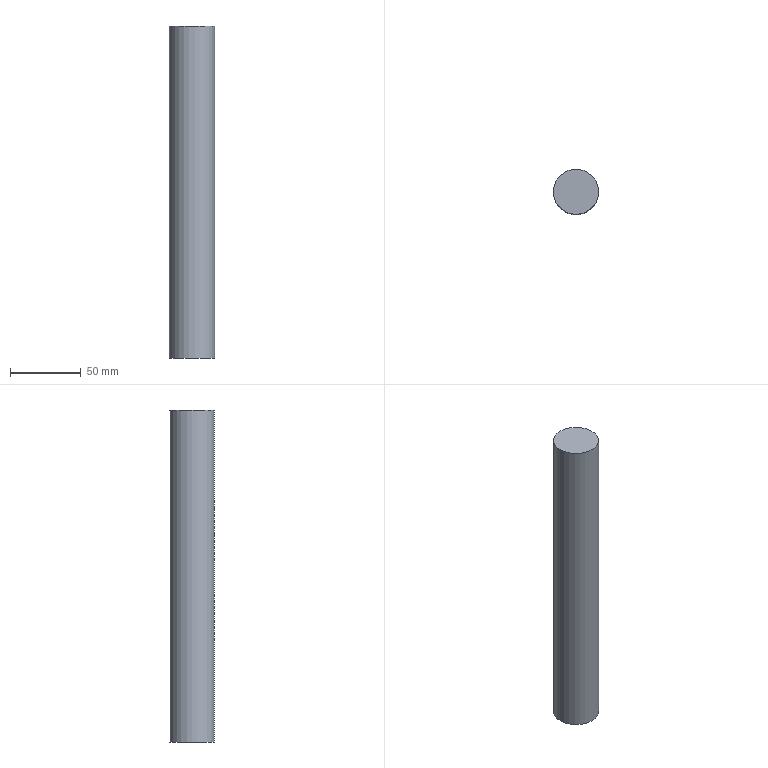Part | NX | features solid 2 | 1 solid | 3 faces | box 32 x 32 x 235 mm | volume 188998 mm3 | plane 2 | cylinder 1 | commonest cylinder face diameters 32 x1
STEP:
#1=CARTESIAN_POINT('',(16.,-155.,-280.));
#2=VERTEX_POINT('',#1);
#3=CARTESIAN_POINT('',(0.,-155.,-280.));
#4=DIRECTION('',(0.,0.,1.));
#5=DIRECTION('',(1.,0.,0.));
#6=AXIS2_PLACEMENT_3D('',#3,#4,#5);
#7=CIRCLE('',#6,16.);
#8=EDGE_CURVE('',#2,#2,#7,.T.);
#9=ORIENTED_EDGE('',*,*,#8,.T.);
#10=EDGE_LOOP('',(#9));
#11=FACE_BOUND('',#10,.T.);
#12=CARTESIAN_POINT('',(16.,-155.,-45.));
#13=VERTEX_POINT('',#12);
#14=CARTESIAN_POINT('',(0.,-155.,-45.));
#15=DIRECTION('',(0.,0.,1.));
#16=DIRECTION('',(1.,0.,0.));
#17=AXIS2_PLACEMENT_3D('',#14,#15,#16);
#18=CIRCLE('',#17,16.);
#19=EDGE_CURVE('',#13,#13,#18,.T.);
#20=ORIENTED_EDGE('',*,*,#19,.F.);
#21=EDGE_LOOP('',(#20));
#22=FACE_BOUND('',#21,.T.);
#23=CARTESIAN_POINT('',(0.,-155.,-280.));
#24=DIRECTION('',(0.,0.,1.));
#25=DIRECTION('',(1.,0.,0.));
#26=AXIS2_PLACEMENT_3D('',#23,#24,#25);
#27=CYLINDRICAL_SURFACE('',#26,16.);
#28=ADVANCED_FACE('',(#11,#22),#27,.T.);
#29=ORIENTED_EDGE('',*,*,#8,.F.);
#30=EDGE_LOOP('',(#29));
#31=FACE_BOUND('',#30,.T.);
#32=CARTESIAN_POINT('',(0.,-155.,-280.));
#33=DIRECTION('',(0.,0.,1.));
#34=DIRECTION('',(1.,0.,0.));
#35=AXIS2_PLACEMENT_3D('',#32,#33,#34);
#36=PLANE('',#35);
#37=ADVANCED_FACE('',(#31),#36,.F.);
#38=ORIENTED_EDGE('',*,*,#19,.T.);
#39=EDGE_LOOP('',(#38));
#40=FACE_BOUND('',#39,.T.);
#41=CARTESIAN_POINT('',(0.,-155.,-45.));
#42=DIRECTION('',(0.,0.,1.));
#43=DIRECTION('',(1.,0.,0.));
#44=AXIS2_PLACEMENT_3D('',#41,#42,#43);
#45=PLANE('',#44);
#46=ADVANCED_FACE('',(#40),#45,.T.);
#47=CLOSED_SHELL('',(#28,#37,#46));
#48=MANIFOLD_SOLID_BREP('',#47);
#49=(LENGTH_UNIT()NAMED_UNIT(*)SI_UNIT(.MILLI.,.METRE.));
#50=UNCERTAINTY_MEASURE_WITH_UNIT(LENGTH_MEASURE(0.00001),#49,'','');
#51=(NAMED_UNIT(*)PLANE_ANGLE_UNIT()SI_UNIT($,.RADIAN.));
#52=(NAMED_UNIT(*)SI_UNIT($,.STERADIAN.)SOLID_ANGLE_UNIT());
#53=(GEOMETRIC_REPRESENTATION_CONTEXT(3)GLOBAL_UNCERTAINTY_ASSIGNED_CONTEXT((#50))GLOBAL_UNIT_ASSIGNED_CONTEXT((#49,#51,#52))REPRESENTATION_CONTEXT('',''));
#54=ADVANCED_BREP_SHAPE_REPRESENTATION('',(#48),#53);